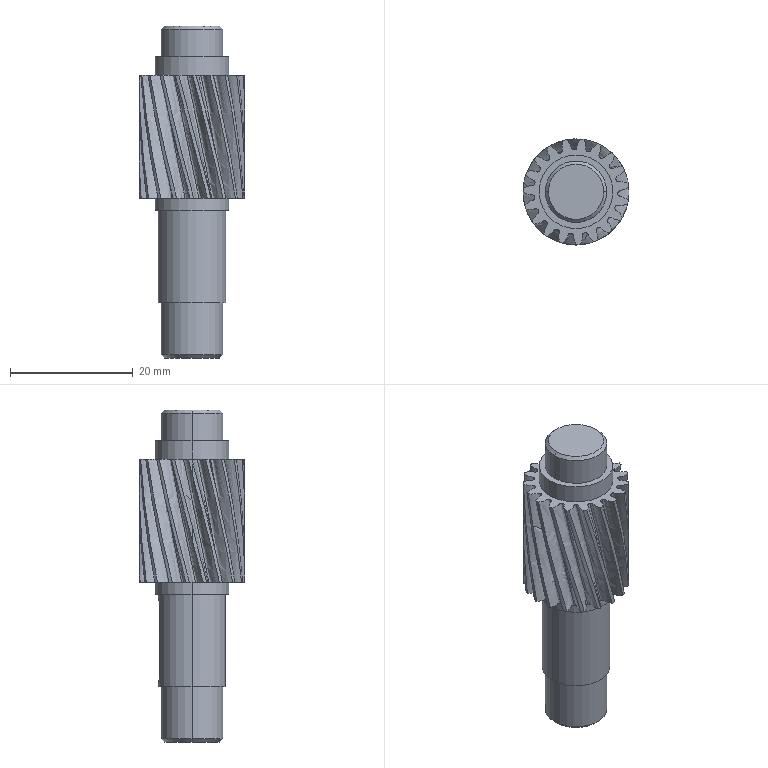Part | SolidWorks | features ICE 6, Chamfer 1, CirPattern 1, Extrusion 1, Helix 1, RefAxis 1, SweepCut 1 | 1 solid | 86 faces | box 17.234 x 17.234 x 54 mm | volume 6790 mm3 | spline 38 | cylinder 34 | plane 10 | cone 4 | commonest cylinder face diameters 17.234 x21 10 x4 12 x4 3 x3 11 x2